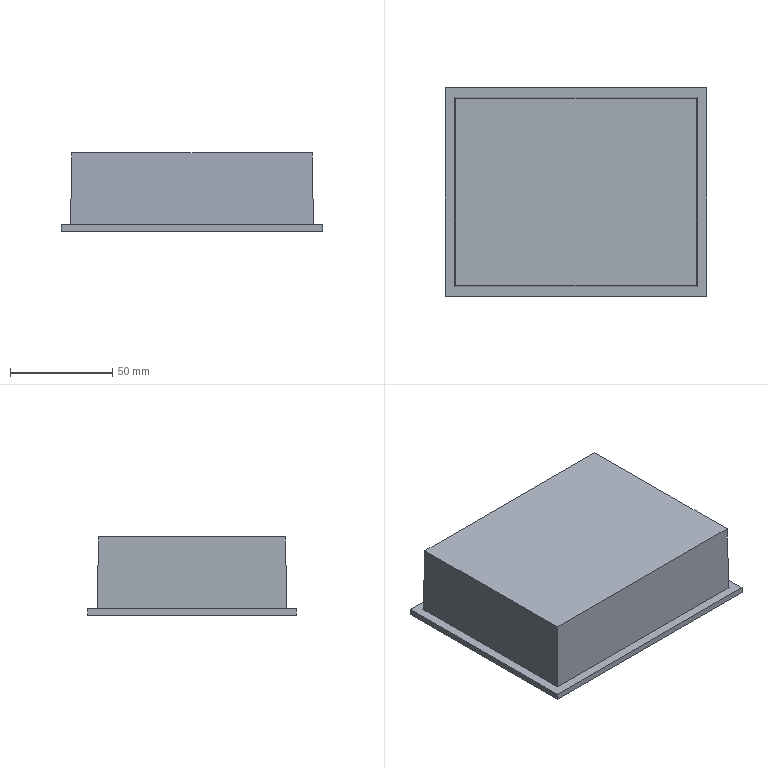Part | STEP file | Touch screen | 1 solid | 16 faces | box 128 x 102 x 38.25 mm | volume 419545 mm3 | plane 16
STEP:
#1=CARTESIAN_POINT('',(0.,0.,0.));
#2=DIRECTION('',(0.,0.,1.));
#3=DIRECTION('',(1.,0.,0.));
#4=AXIS2_PLACEMENT_3D('',#1,#2,#3);
#5=CARTESIAN_POINT('',(-64.,51.,0.));
#6=VERTEX_POINT('',#5);
#7=CARTESIAN_POINT('',(-64.,-51.,0.));
#8=VERTEX_POINT('',#7);
#9=CARTESIAN_POINT('',(-64.,51.,0.));
#10=DIRECTION('',(0.,-1.,0.));
#11=VECTOR('',#10,1.);
#12=LINE('',#9,#11);
#13=CARTESIAN_POINT('',(-64.,51.,3.));
#14=DIRECTION('',(1.,0.,0.));
#15=DIRECTION('',(0.,1.,0.));
#16=AXIS2_PLACEMENT_3D('',#13,#14,#15);
#17=PLANE('',#16);
#18=CARTESIAN_POINT('',(0.,-3.));
#19=DIRECTION('',(-1.,0.));
#20=VECTOR('',#19,1.);
#21=LINE('',#18,#20);
#22=(GEOMETRIC_REPRESENTATION_CONTEXT(2)PARAMETRIC_REPRESENTATION_CONTEXT()REPRESENTATION_CONTEXT('',''));
#23=DEFINITIONAL_REPRESENTATION('',(#21),#22);
#24=PCURVE('',#17,#23);
#25=CARTESIAN_POINT('',(0.,0.,0.));
#26=DIRECTION('',(0.,0.,-1.));
#27=DIRECTION('',(-1.,0.,0.));
#28=AXIS2_PLACEMENT_3D('',#25,#26,#27);
#29=PLANE('',#28);
#30=CARTESIAN_POINT('',(64.,51.));
#31=DIRECTION('',(0.,-1.));
#32=VECTOR('',#31,1.);
#33=LINE('',#30,#32);
#34=(GEOMETRIC_REPRESENTATION_CONTEXT(2)PARAMETRIC_REPRESENTATION_CONTEXT()REPRESENTATION_CONTEXT('',''));
#35=DEFINITIONAL_REPRESENTATION('',(#33),#34);
#36=PCURVE('',#29,#35);
#37=SURFACE_CURVE('',#12,(#24,#36),.PCURVE_S1.);
#38=EDGE_CURVE('',#6,#8,#37,.T.);
#39=ORIENTED_EDGE('',*,*,#38,.T.);
#40=CARTESIAN_POINT('',(-64.,-51.,3.));
#41=VERTEX_POINT('',#40);
#42=CARTESIAN_POINT('',(-64.,-51.,3.));
#43=DIRECTION('',(0.,0.,-1.));
#44=VECTOR('',#43,1.);
#45=LINE('',#42,#44);
#46=CARTESIAN_POINT('',(-102.,0.));
#47=DIRECTION('',(0.,-1.));
#48=VECTOR('',#47,1.);
#49=LINE('',#46,#48);
#50=(GEOMETRIC_REPRESENTATION_CONTEXT(2)PARAMETRIC_REPRESENTATION_CONTEXT()REPRESENTATION_CONTEXT('',''));
#51=DEFINITIONAL_REPRESENTATION('',(#49),#50);
#52=PCURVE('',#17,#51);
#53=CARTESIAN_POINT('',(64.,-51.,3.));
#54=DIRECTION('',(0.,1.,0.));
#55=DIRECTION('',(-1.,0.,0.));
#56=AXIS2_PLACEMENT_3D('',#53,#54,#55);
#57=PLANE('',#56);
#58=CARTESIAN_POINT('',(128.,0.));
#59=DIRECTION('',(0.,-1.));
#60=VECTOR('',#59,1.);
#61=LINE('',#58,#60);
#62=(GEOMETRIC_REPRESENTATION_CONTEXT(2)PARAMETRIC_REPRESENTATION_CONTEXT()REPRESENTATION_CONTEXT('',''));
#63=DEFINITIONAL_REPRESENTATION('',(#61),#62);
#64=PCURVE('',#57,#63);
#65=SURFACE_CURVE('',#45,(#52,#64),.PCURVE_S1.);
#66=EDGE_CURVE('',#41,#8,#65,.T.);
#67=ORIENTED_EDGE('',*,*,#66,.F.);
#68=CARTESIAN_POINT('',(-64.,51.,3.));
#69=VERTEX_POINT('',#68);
#70=CARTESIAN_POINT('',(-64.,51.,3.));
#71=DIRECTION('',(0.,-1.,0.));
#72=VECTOR('',#71,1.);
#73=LINE('',#70,#72);
#74=CARTESIAN_POINT('',(0.,0.));
#75=DIRECTION('',(-1.,0.));
#76=VECTOR('',#75,1.);
#77=LINE('',#74,#76);
#78=(GEOMETRIC_REPRESENTATION_CONTEXT(2)PARAMETRIC_REPRESENTATION_CONTEXT()REPRESENTATION_CONTEXT('',''));
#79=DEFINITIONAL_REPRESENTATION('',(#77),#78);
#80=PCURVE('',#17,#79);
#81=CARTESIAN_POINT('',(0.,0.,3.));
#82=DIRECTION('',(0.,0.,-1.));
#83=DIRECTION('',(-1.,0.,0.));
#84=AXIS2_PLACEMENT_3D('',#81,#82,#83);
#85=PLANE('',#84);
#86=CARTESIAN_POINT('',(64.,51.));
#87=DIRECTION('',(0.,-1.));
#88=VECTOR('',#87,1.);
#89=LINE('',#86,#88);
#90=(GEOMETRIC_REPRESENTATION_CONTEXT(2)PARAMETRIC_REPRESENTATION_CONTEXT()REPRESENTATION_CONTEXT('',''));
#91=DEFINITIONAL_REPRESENTATION('',(#89),#90);
#92=PCURVE('',#85,#91);
#93=SURFACE_CURVE('',#73,(#80,#92),.PCURVE_S1.);
#94=EDGE_CURVE('',#69,#41,#93,.T.);
#95=ORIENTED_EDGE('',*,*,#94,.F.);
#96=CARTESIAN_POINT('',(-64.,51.,3.));
#97=DIRECTION('',(0.,0.,-1.));
#98=VECTOR('',#97,1.);
#99=LINE('',#96,#98);
#100=CARTESIAN_POINT('',(0.,0.));
#101=DIRECTION('',(0.,-1.));
#102=VECTOR('',#101,1.);
#103=LINE('',#100,#102);
#104=(GEOMETRIC_REPRESENTATION_CONTEXT(2)PARAMETRIC_REPRESENTATION_CONTEXT()REPRESENTATION_CONTEXT('',''));
#105=DEFINITIONAL_REPRESENTATION('',(#103),#104);
#106=PCURVE('',#17,#105);
#107=CARTESIAN_POINT('',(64.,51.,3.));
#108=DIRECTION('',(0.,-1.,0.));
#109=DIRECTION('',(1.,0.,0.));
#110=AXIS2_PLACEMENT_3D('',#107,#108,#109);
#111=PLANE('',#110);
#112=CARTESIAN_POINT('',(-128.,0.));
#113=DIRECTION('',(0.,-1.));
#114=VECTOR('',#113,1.);
#115=LINE('',#112,#114);
#116=(GEOMETRIC_REPRESENTATION_CONTEXT(2)PARAMETRIC_REPRESENTATION_CONTEXT()REPRESENTATION_CONTEXT('',''));
#117=DEFINITIONAL_REPRESENTATION('',(#115),#116);
#118=PCURVE('',#111,#117);
#119=SURFACE_CURVE('',#99,(#106,#118),.PCURVE_S1.);
#120=EDGE_CURVE('',#69,#6,#119,.T.);
#121=ORIENTED_EDGE('',*,*,#120,.T.);
#122=EDGE_LOOP('',(#39,#67,#95,#121));
#123=FACE_BOUND('',#122,.T.);
#124=ADVANCED_FACE('',(#123),#17,.F.);
#125=CARTESIAN_POINT('',(64.,-51.,0.));
#126=VERTEX_POINT('',#125);
#127=CARTESIAN_POINT('',(64.,-51.,0.));
#128=DIRECTION('',(1.,0.,0.));
#129=VECTOR('',#128,1.);
#130=LINE('',#127,#129);
#131=CARTESIAN_POINT('',(0.,-3.));
#132=DIRECTION('',(-1.,0.));
#133=VECTOR('',#132,1.);
#134=LINE('',#131,#133);
#135=(GEOMETRIC_REPRESENTATION_CONTEXT(2)PARAMETRIC_REPRESENTATION_CONTEXT()REPRESENTATION_CONTEXT('',''));
#136=DEFINITIONAL_REPRESENTATION('',(#134),#135);
#137=PCURVE('',#57,#136);
#138=CARTESIAN_POINT('',(-64.,-51.));
#139=DIRECTION('',(-1.,0.));
#140=VECTOR('',#139,1.);
#141=LINE('',#138,#140);
#142=(GEOMETRIC_REPRESENTATION_CONTEXT(2)PARAMETRIC_REPRESENTATION_CONTEXT()REPRESENTATION_CONTEXT('',''));
#143=DEFINITIONAL_REPRESENTATION('',(#141),#142);
#144=PCURVE('',#29,#143);
#145=SURFACE_CURVE('',#130,(#137,#144),.PCURVE_S1.);
#146=EDGE_CURVE('',#8,#126,#145,.T.);
#147=ORIENTED_EDGE('',*,*,#146,.T.);
#148=CARTESIAN_POINT('',(64.,-51.,3.));
#149=VERTEX_POINT('',#148);
#150=CARTESIAN_POINT('',(64.,-51.,3.));
#151=DIRECTION('',(0.,0.,-1.));
#152=VECTOR('',#151,1.);
#153=LINE('',#150,#152);
#154=CARTESIAN_POINT('',(0.,0.));
#155=DIRECTION('',(0.,-1.));
#156=VECTOR('',#155,1.);
#157=LINE('',#154,#156);
#158=(GEOMETRIC_REPRESENTATION_CONTEXT(2)PARAMETRIC_REPRESENTATION_CONTEXT()REPRESENTATION_CONTEXT('',''));
#159=DEFINITIONAL_REPRESENTATION('',(#157),#158);
#160=PCURVE('',#57,#159);
#161=CARTESIAN_POINT('',(64.,51.,3.));
#162=DIRECTION('',(-1.,0.,0.));
#163=DIRECTION('',(0.,-1.,0.));
#164=AXIS2_PLACEMENT_3D('',#161,#162,#163);
#165=PLANE('',#164);
#166=CARTESIAN_POINT('',(102.,0.));
#167=DIRECTION('',(0.,-1.));
#168=VECTOR('',#167,1.);
#169=LINE('',#166,#168);
#170=(GEOMETRIC_REPRESENTATION_CONTEXT(2)PARAMETRIC_REPRESENTATION_CONTEXT()REPRESENTATION_CONTEXT('',''));
#171=DEFINITIONAL_REPRESENTATION('',(#169),#170);
#172=PCURVE('',#165,#171);
#173=SURFACE_CURVE('',#153,(#160,#172),.PCURVE_S1.);
#174=EDGE_CURVE('',#149,#126,#173,.T.);
#175=ORIENTED_EDGE('',*,*,#174,.F.);
#176=CARTESIAN_POINT('',(64.,-51.,3.));
#177=DIRECTION('',(1.,0.,0.));
#178=VECTOR('',#177,1.);
#179=LINE('',#176,#178);
#180=CARTESIAN_POINT('',(0.,0.));
#181=DIRECTION('',(-1.,0.));
#182=VECTOR('',#181,1.);
#183=LINE('',#180,#182);
#184=(GEOMETRIC_REPRESENTATION_CONTEXT(2)PARAMETRIC_REPRESENTATION_CONTEXT()REPRESENTATION_CONTEXT('',''));
#185=DEFINITIONAL_REPRESENTATION('',(#183),#184);
#186=PCURVE('',#57,#185);
#187=CARTESIAN_POINT('',(-64.,-51.));
#188=DIRECTION('',(-1.,0.));
#189=VECTOR('',#188,1.);
#190=LINE('',#187,#189);
#191=(GEOMETRIC_REPRESENTATION_CONTEXT(2)PARAMETRIC_REPRESENTATION_CONTEXT()REPRESENTATION_CONTEXT('',''));
#192=DEFINITIONAL_REPRESENTATION('',(#190),#191);
#193=PCURVE('',#85,#192);
#194=SURFACE_CURVE('',#179,(#186,#193),.PCURVE_S1.);
#195=EDGE_CURVE('',#41,#149,#194,.T.);
#196=ORIENTED_EDGE('',*,*,#195,.F.);
#197=ORIENTED_EDGE('',*,*,#66,.T.);
#198=EDGE_LOOP('',(#147,#175,#196,#197));
#199=FACE_BOUND('',#198,.T.);
#200=ADVANCED_FACE('',(#199),#57,.F.);
#201=CARTESIAN_POINT('',(64.,51.,0.));
#202=VERTEX_POINT('',#201);
#203=CARTESIAN_POINT('',(64.,51.,0.));
#204=DIRECTION('',(0.,1.,0.));
#205=VECTOR('',#204,1.);
#206=LINE('',#203,#205);
#207=CARTESIAN_POINT('',(0.,-3.));
#208=DIRECTION('',(-1.,0.));
#209=VECTOR('',#208,1.);
#210=LINE('',#207,#209);
#211=(GEOMETRIC_REPRESENTATION_CONTEXT(2)PARAMETRIC_REPRESENTATION_CONTEXT()REPRESENTATION_CONTEXT('',''));
#212=DEFINITIONAL_REPRESENTATION('',(#210),#211);
#213=PCURVE('',#165,#212);
#214=CARTESIAN_POINT('',(-64.,51.));
#215=DIRECTION('',(0.,1.));
#216=VECTOR('',#215,1.);
#217=LINE('',#214,#216);
#218=(GEOMETRIC_REPRESENTATION_CONTEXT(2)PARAMETRIC_REPRESENTATION_CONTEXT()REPRESENTATION_CONTEXT('',''));
#219=DEFINITIONAL_REPRESENTATION('',(#217),#218);
#220=PCURVE('',#29,#219);
#221=SURFACE_CURVE('',#206,(#213,#220),.PCURVE_S1.);
#222=EDGE_CURVE('',#126,#202,#221,.T.);
#223=ORIENTED_EDGE('',*,*,#222,.T.);
#224=CARTESIAN_POINT('',(64.,51.,3.));
#225=VERTEX_POINT('',#224);
#226=CARTESIAN_POINT('',(64.,51.,3.));
#227=DIRECTION('',(0.,0.,-1.));
#228=VECTOR('',#227,1.);
#229=LINE('',#226,#228);
#230=CARTESIAN_POINT('',(0.,0.));
#231=DIRECTION('',(0.,-1.));
#232=VECTOR('',#231,1.);
#233=LINE('',#230,#232);
#234=(GEOMETRIC_REPRESENTATION_CONTEXT(2)PARAMETRIC_REPRESENTATION_CONTEXT()REPRESENTATION_CONTEXT('',''));
#235=DEFINITIONAL_REPRESENTATION('',(#233),#234);
#236=PCURVE('',#165,#235);
#237=CARTESIAN_POINT('',(0.,0.));
#238=DIRECTION('',(0.,-1.));
#239=VECTOR('',#238,1.);
#240=LINE('',#237,#239);
#241=(GEOMETRIC_REPRESENTATION_CONTEXT(2)PARAMETRIC_REPRESENTATION_CONTEXT()REPRESENTATION_CONTEXT('',''));
#242=DEFINITIONAL_REPRESENTATION('',(#240),#241);
#243=PCURVE('',#111,#242);
#244=SURFACE_CURVE('',#229,(#236,#243),.PCURVE_S1.);
#245=EDGE_CURVE('',#225,#202,#244,.T.);
#246=ORIENTED_EDGE('',*,*,#245,.F.);
#247=CARTESIAN_POINT('',(64.,51.,3.));
#248=DIRECTION('',(0.,1.,0.));
#249=VECTOR('',#248,1.);
#250=LINE('',#247,#249);
#251=CARTESIAN_POINT('',(0.,0.));
#252=DIRECTION('',(-1.,0.));
#253=VECTOR('',#252,1.);
#254=LINE('',#251,#253);
#255=(GEOMETRIC_REPRESENTATION_CONTEXT(2)PARAMETRIC_REPRESENTATION_CONTEXT()REPRESENTATION_CONTEXT('',''));
#256=DEFINITIONAL_REPRESENTATION('',(#254),#255);
#257=PCURVE('',#165,#256);
#258=CARTESIAN_POINT('',(-64.,51.));
#259=DIRECTION('',(0.,1.));
#260=VECTOR('',#259,1.);
#261=LINE('',#258,#260);
#262=(GEOMETRIC_REPRESENTATION_CONTEXT(2)PARAMETRIC_REPRESENTATION_CONTEXT()REPRESENTATION_CONTEXT('',''));
#263=DEFINITIONAL_REPRESENTATION('',(#261),#262);
#264=PCURVE('',#85,#263);
#265=SURFACE_CURVE('',#250,(#257,#264),.PCURVE_S1.);
#266=EDGE_CURVE('',#149,#225,#265,.T.);
#267=ORIENTED_EDGE('',*,*,#266,.F.);
#268=ORIENTED_EDGE('',*,*,#174,.T.);
#269=EDGE_LOOP('',(#223,#246,#267,#268));
#270=FACE_BOUND('',#269,.T.);
#271=ADVANCED_FACE('',(#270),#165,.F.);
#272=CARTESIAN_POINT('',(64.,51.,0.));
#273=DIRECTION('',(-1.,0.,0.));
#274=VECTOR('',#273,1.);
#275=LINE('',#272,#274);
#276=CARTESIAN_POINT('',(0.,-3.));
#277=DIRECTION('',(-1.,0.));
#278=VECTOR('',#277,1.);
#279=LINE('',#276,#278);
#280=(GEOMETRIC_REPRESENTATION_CONTEXT(2)PARAMETRIC_REPRESENTATION_CONTEXT()REPRESENTATION_CONTEXT('',''));
#281=DEFINITIONAL_REPRESENTATION('',(#279),#280);
#282=PCURVE('',#111,#281);
#283=CARTESIAN_POINT('',(-64.,51.));
#284=DIRECTION('',(1.,0.));
#285=VECTOR('',#284,1.);
#286=LINE('',#283,#285);
#287=(GEOMETRIC_REPRESENTATION_CONTEXT(2)PARAMETRIC_REPRESENTATION_CONTEXT()REPRESENTATION_CONTEXT('',''));
#288=DEFINITIONAL_REPRESENTATION('',(#286),#287);
#289=PCURVE('',#29,#288);
#290=SURFACE_CURVE('',#275,(#282,#289),.PCURVE_S1.);
#291=EDGE_CURVE('',#202,#6,#290,.T.);
#292=ORIENTED_EDGE('',*,*,#291,.T.);
#293=ORIENTED_EDGE('',*,*,#120,.F.);
#294=CARTESIAN_POINT('',(64.,51.,3.));
#295=DIRECTION('',(-1.,0.,0.));
#296=VECTOR('',#295,1.);
#297=LINE('',#294,#296);
#298=CARTESIAN_POINT('',(0.,0.));
#299=DIRECTION('',(-1.,0.));
#300=VECTOR('',#299,1.);
#301=LINE('',#298,#300);
#302=(GEOMETRIC_REPRESENTATION_CONTEXT(2)PARAMETRIC_REPRESENTATION_CONTEXT()REPRESENTATION_CONTEXT('',''));
#303=DEFINITIONAL_REPRESENTATION('',(#301),#302);
#304=PCURVE('',#111,#303);
#305=CARTESIAN_POINT('',(-64.,51.));
#306=DIRECTION('',(1.,0.));
#307=VECTOR('',#306,1.);
#308=LINE('',#305,#307);
#309=(GEOMETRIC_REPRESENTATION_CONTEXT(2)PARAMETRIC_REPRESENTATION_CONTEXT()REPRESENTATION_CONTEXT('',''));
#310=DEFINITIONAL_REPRESENTATION('',(#308),#309);
#311=PCURVE('',#85,#310);
#312=SURFACE_CURVE('',#297,(#304,#311),.PCURVE_S1.);
#313=EDGE_CURVE('',#225,#69,#312,.T.);
#314=ORIENTED_EDGE('',*,*,#313,.F.);
#315=ORIENTED_EDGE('',*,*,#245,.T.);
#316=EDGE_LOOP('',(#292,#293,#314,#315));
#317=FACE_BOUND('',#316,.T.);
#318=ADVANCED_FACE('',(#317),#111,.F.);
#319=CARTESIAN_POINT('',(-59.5,-46.5,3.));
#320=VERTEX_POINT('',#319);
#321=CARTESIAN_POINT('',(59.5,-46.5,3.));
#322=VERTEX_POINT('',#321);
#323=CARTESIAN_POINT('',(59.5,-46.5,3.));
#324=DIRECTION('',(1.,0.,0.));
#325=VECTOR('',#324,1.);
#326=LINE('',#323,#325);
#327=CARTESIAN_POINT('',(-59.5,-46.5));
#328=DIRECTION('',(-1.,0.));
#329=VECTOR('',#328,1.);
#330=LINE('',#327,#329);
#331=(GEOMETRIC_REPRESENTATION_CONTEXT(2)PARAMETRIC_REPRESENTATION_CONTEXT()REPRESENTATION_CONTEXT('',''));
#332=DEFINITIONAL_REPRESENTATION('',(#330),#331);
#333=PCURVE('',#85,#332);
#334=CARTESIAN_POINT('',(0.,-46.542,0.9705));
#335=DIRECTION('',(0.,-0.9998,0.02085));
#336=DIRECTION('',(0.,-0.02085,-0.9998));
#337=AXIS2_PLACEMENT_3D('',#334,#335,#336);
#338=PLANE('',#337);
#339=CARTESIAN_POINT('',(-2.03,59.5));
#340=DIRECTION('',(0.,1.));
#341=VECTOR('',#340,1.);
#342=LINE('',#339,#341);
#343=(GEOMETRIC_REPRESENTATION_CONTEXT(2)PARAMETRIC_REPRESENTATION_CONTEXT()REPRESENTATION_CONTEXT('',''));
#344=DEFINITIONAL_REPRESENTATION('',(#342),#343);
#345=PCURVE('',#338,#344);
#346=SURFACE_CURVE('',#326,(#333,#345),.PCURVE_S1.);
#347=EDGE_CURVE('',#320,#322,#346,.T.);
#348=ORIENTED_EDGE('',*,*,#347,.F.);
#349=CARTESIAN_POINT('',(-59.5,46.5,3.));
#350=VERTEX_POINT('',#349);
#351=CARTESIAN_POINT('',(-59.5,46.5,3.));
#352=DIRECTION('',(0.,-1.,0.));
#353=VECTOR('',#352,1.);
#354=LINE('',#351,#353);
#355=CARTESIAN_POINT('',(59.5,46.5));
#356=DIRECTION('',(0.,-1.));
#357=VECTOR('',#356,1.);
#358=LINE('',#355,#357);
#359=(GEOMETRIC_REPRESENTATION_CONTEXT(2)PARAMETRIC_REPRESENTATION_CONTEXT()REPRESENTATION_CONTEXT('',''));
#360=DEFINITIONAL_REPRESENTATION('',(#358),#359);
#361=PCURVE('',#85,#360);
#362=CARTESIAN_POINT('',(-59.535,0.,1.072));
#363=DIRECTION('',(-0.9998,0.,0.01801));
#364=DIRECTION('',(0.01801,0.,0.9998));
#365=AXIS2_PLACEMENT_3D('',#362,#363,#364);
#366=PLANE('',#365);
#367=CARTESIAN_POINT('',(1.928,46.5));
#368=DIRECTION('',(0.,-1.));
#369=VECTOR('',#368,1.);
#370=LINE('',#367,#369);
#371=(GEOMETRIC_REPRESENTATION_CONTEXT(2)PARAMETRIC_REPRESENTATION_CONTEXT()REPRESENTATION_CONTEXT('',''));
#372=DEFINITIONAL_REPRESENTATION('',(#370),#371);
#373=PCURVE('',#366,#372);
#374=SURFACE_CURVE('',#354,(#361,#373),.PCURVE_S1.);
#375=EDGE_CURVE('',#350,#320,#374,.T.);
#376=ORIENTED_EDGE('',*,*,#375,.F.);
#377=CARTESIAN_POINT('',(59.5,46.5,3.));
#378=VERTEX_POINT('',#377);
#379=CARTESIAN_POINT('',(59.5,46.5,3.));
#380=DIRECTION('',(-1.,0.,0.));
#381=VECTOR('',#380,1.);
#382=LINE('',#379,#381);
#383=CARTESIAN_POINT('',(-59.5,46.5));
#384=DIRECTION('',(1.,0.));
#385=VECTOR('',#384,1.);
#386=LINE('',#383,#385);
#387=(GEOMETRIC_REPRESENTATION_CONTEXT(2)PARAMETRIC_REPRESENTATION_CONTEXT()REPRESENTATION_CONTEXT('',''));
#388=DEFINITIONAL_REPRESENTATION('',(#386),#387);
#389=PCURVE('',#85,#388);
#390=CARTESIAN_POINT('',(0.,46.542,0.9705));
#391=DIRECTION('',(0.,0.9998,0.02085));
#392=DIRECTION('',(0.,-0.02085,0.9998));
#393=AXIS2_PLACEMENT_3D('',#390,#391,#392);
#394=PLANE('',#393);
#395=CARTESIAN_POINT('',(2.03,59.5));
#396=DIRECTION('',(0.,-1.));
#397=VECTOR('',#396,1.);
#398=LINE('',#395,#397);
#399=(GEOMETRIC_REPRESENTATION_CONTEXT(2)PARAMETRIC_REPRESENTATION_CONTEXT()REPRESENTATION_CONTEXT('',''));
#400=DEFINITIONAL_REPRESENTATION('',(#398),#399);
#401=PCURVE('',#394,#400);
#402=SURFACE_CURVE('',#382,(#389,#401),.PCURVE_S1.);
#403=EDGE_CURVE('',#378,#350,#402,.T.);
#404=ORIENTED_EDGE('',*,*,#403,.F.);
#405=CARTESIAN_POINT('',(59.5,46.5,3.));
#406=DIRECTION('',(0.,1.,0.));
#407=VECTOR('',#406,1.);
#408=LINE('',#405,#407);
#409=CARTESIAN_POINT('',(-59.5,46.5));
#410=DIRECTION('',(0.,1.));
#411=VECTOR('',#410,1.);
#412=LINE('',#409,#411);
#413=(GEOMETRIC_REPRESENTATION_CONTEXT(2)PARAMETRIC_REPRESENTATION_CONTEXT()REPRESENTATION_CONTEXT('',''));
#414=DEFINITIONAL_REPRESENTATION('',(#412),#413);
#415=PCURVE('',#85,#414);
#416=CARTESIAN_POINT('',(59.535,0.,1.072));
#417=DIRECTION('',(0.9998,0.,0.01801));
#418=DIRECTION('',(0.01801,0.,-0.9998));
#419=AXIS2_PLACEMENT_3D('',#416,#417,#418);
#420=PLANE('',#419);
#421=CARTESIAN_POINT('',(-1.928,46.5));
#422=DIRECTION('',(0.,1.));
#423=VECTOR('',#422,1.);
#424=LINE('',#421,#423);
#425=(GEOMETRIC_REPRESENTATION_CONTEXT(2)PARAMETRIC_REPRESENTATION_CONTEXT()REPRESENTATION_CONTEXT('',''));
#426=DEFINITIONAL_REPRESENTATION('',(#424),#425);
#427=PCURVE('',#420,#426);
#428=SURFACE_CURVE('',#408,(#415,#427),.PCURVE_S1.);
#429=EDGE_CURVE('',#322,#378,#428,.T.);
#430=ORIENTED_EDGE('',*,*,#429,.F.);
#431=EDGE_LOOP('',(#348,#376,#404,#430));
#432=FACE_BOUND('',#431,.T.);
#433=ORIENTED_EDGE('',*,*,#94,.T.);
#434=ORIENTED_EDGE('',*,*,#195,.T.);
#435=ORIENTED_EDGE('',*,*,#266,.T.);
#436=ORIENTED_EDGE('',*,*,#313,.T.);
#437=EDGE_LOOP('',(#433,#434,#435,#436));
#438=FACE_BOUND('',#437,.T.);
#439=ADVANCED_FACE('',(#432,#438),#85,.F.);
#440=CARTESIAN_POINT('',(56.,41.,0.));
#441=VERTEX_POINT('',#440);
#442=CARTESIAN_POINT('',(56.,-41.,0.));
#443=VERTEX_POINT('',#442);
#444=CARTESIAN_POINT('',(56.,41.,0.));
#445=DIRECTION('',(0.,-1.,0.));
#446=VECTOR('',#445,1.);
#447=LINE('',#444,#446);
#448=CARTESIAN_POINT('',(-56.,41.));
#449=DIRECTION('',(0.,-1.));
#450=VECTOR('',#449,1.);
#451=LINE('',#448,#450);
#452=(GEOMETRIC_REPRESENTATION_CONTEXT(2)PARAMETRIC_REPRESENTATION_CONTEXT()REPRESENTATION_CONTEXT('',''));
#453=DEFINITIONAL_REPRESENTATION('',(#451),#452);
#454=PCURVE('',#29,#453);
#455=CARTESIAN_POINT('',(56.,41.,0.5));
#456=DIRECTION('',(1.,0.,0.));
#457=DIRECTION('',(0.,0.,-1.));
#458=AXIS2_PLACEMENT_3D('',#455,#456,#457);
#459=PLANE('',#458);
#460=CARTESIAN_POINT('',(0.5,0.));
#461=DIRECTION('',(0.,-1.));
#462=VECTOR('',#461,1.);
#463=LINE('',#460,#462);
#464=(GEOMETRIC_REPRESENTATION_CONTEXT(2)PARAMETRIC_REPRESENTATION_CONTEXT()REPRESENTATION_CONTEXT('',''));
#465=DEFINITIONAL_REPRESENTATION('',(#463),#464);
#466=PCURVE('',#459,#465);
#467=SURFACE_CURVE('',#447,(#454,#466),.PCURVE_S1.);
#468=EDGE_CURVE('',#441,#443,#467,.T.);
#469=ORIENTED_EDGE('',*,*,#468,.F.);
#470=CARTESIAN_POINT('',(-56.,41.,0.));
#471=VERTEX_POINT('',#470);
#472=CARTESIAN_POINT('',(-56.,41.,0.));
#473=DIRECTION('',(1.,0.,0.));
#474=VECTOR('',#473,1.);
#475=LINE('',#472,#474);
#476=CARTESIAN_POINT('',(56.,41.));
#477=DIRECTION('',(-1.,0.));
#478=VECTOR('',#477,1.);
#479=LINE('',#476,#478);
#480=(GEOMETRIC_REPRESENTATION_CONTEXT(2)PARAMETRIC_REPRESENTATION_CONTEXT()REPRESENTATION_CONTEXT('',''));
#481=DEFINITIONAL_REPRESENTATION('',(#479),#480);
#482=PCURVE('',#29,#481);
#483=CARTESIAN_POINT('',(-56.,41.,0.5));
#484=DIRECTION('',(0.,1.,0.));
#485=DIRECTION('',(0.,0.,1.));
#486=AXIS2_PLACEMENT_3D('',#483,#484,#485);
#487=PLANE('',#486);
#488=CARTESIAN_POINT('',(-0.5,0.));
#489=DIRECTION('',(0.,1.));
#490=VECTOR('',#489,1.);
#491=LINE('',#488,#490);
#492=(GEOMETRIC_REPRESENTATION_CONTEXT(2)PARAMETRIC_REPRESENTATION_CONTEXT()REPRESENTATION_CONTEXT('',''));
#493=DEFINITIONAL_REPRESENTATION('',(#491),#492);
#494=PCURVE('',#487,#493);
#495=SURFACE_CURVE('',#475,(#482,#494),.PCURVE_S1.);
#496=EDGE_CURVE('',#471,#441,#495,.T.);
#497=ORIENTED_EDGE('',*,*,#496,.F.);
#498=CARTESIAN_POINT('',(-56.,-41.,0.));
#499=VERTEX_POINT('',#498);
#500=CARTESIAN_POINT('',(-56.,41.,0.));
#501=DIRECTION('',(0.,1.,0.));
#502=VECTOR('',#501,1.);
#503=LINE('',#500,#502);
#504=CARTESIAN_POINT('',(56.,41.));
#505=DIRECTION('',(0.,1.));
#506=VECTOR('',#505,1.);
#507=LINE('',#504,#506);
#508=(GEOMETRIC_REPRESENTATION_CONTEXT(2)PARAMETRIC_REPRESENTATION_CONTEXT()REPRESENTATION_CONTEXT('',''));
#509=DEFINITIONAL_REPRESENTATION('',(#507),#508);
#510=PCURVE('',#29,#509);
#511=CARTESIAN_POINT('',(-56.,41.,0.5));
#512=DIRECTION('',(-1.,0.,0.));
#513=DIRECTION('',(0.,0.,1.));
#514=AXIS2_PLACEMENT_3D('',#511,#512,#513);
#515=PLANE('',#514);
#516=CARTESIAN_POINT('',(-0.5,0.));
#517=DIRECTION('',(0.,1.));
#518=VECTOR('',#517,1.);
#519=LINE('',#516,#518);
#520=(GEOMETRIC_REPRESENTATION_CONTEXT(2)PARAMETRIC_REPRESENTATION_CONTEXT()REPRESENTATION_CONTEXT('',''));
#521=DEFINITIONAL_REPRESENTATION('',(#519),#520);
#522=PCURVE('',#515,#521);
#523=SURFACE_CURVE('',#503,(#510,#522),.PCURVE_S1.);
#524=EDGE_CURVE('',#499,#471,#523,.T.);
#525=ORIENTED_EDGE('',*,*,#524,.F.);
#526=CARTESIAN_POINT('',(-56.,-41.,0.));
#527=DIRECTION('',(-1.,0.,0.));
#528=VECTOR('',#527,1.);
#529=LINE('',#526,#528);
#530=CARTESIAN_POINT('',(56.,-41.));
#531=DIRECTION('',(1.,0.));
#532=VECTOR('',#531,1.);
#533=LINE('',#530,#532);
#534=(GEOMETRIC_REPRESENTATION_CONTEXT(2)PARAMETRIC_REPRESENTATION_CONTEXT()REPRESENTATION_CONTEXT('',''));
#535=DEFINITIONAL_REPRESENTATION('',(#533),#534);
#536=PCURVE('',#29,#535);
#537=CARTESIAN_POINT('',(-56.,-41.,0.5));
#538=DIRECTION('',(0.,-1.,0.));
#539=DIRECTION('',(0.,0.,-1.));
#540=AXIS2_PLACEMENT_3D('',#537,#538,#539);
#541=PLANE('',#540);
#542=CARTESIAN_POINT('',(0.5,0.));
#543=DIRECTION('',(0.,-1.));
#544=VECTOR('',#543,1.);
#545=LINE('',#542,#544);
#546=(GEOMETRIC_REPRESENTATION_CONTEXT(2)PARAMETRIC_REPRESENTATION_CONTEXT()REPRESENTATION_CONTEXT('',''));
#547=DEFINITIONAL_REPRESENTATION('',(#545),#546);
#548=PCURVE('',#541,#547);
#549=SURFACE_CURVE('',#529,(#536,#548),.PCURVE_S1.);
#550=EDGE_CURVE('',#443,#499,#549,.T.);
#551=ORIENTED_EDGE('',*,*,#550,.F.);
#552=EDGE_LOOP('',(#469,#497,#525,#551));
#553=FACE_BOUND('',#552,.T.);
#554=ORIENTED_EDGE('',*,*,#38,.F.);
#555=ORIENTED_EDGE('',*,*,#291,.F.);
#556=ORIENTED_EDGE('',*,*,#222,.F.);
#557=ORIENTED_EDGE('',*,*,#146,.F.);
#558=EDGE_LOOP('',(#554,#555,#556,#557));
#559=FACE_BOUND('',#558,.T.);
#560=ADVANCED_FACE('',(#553,#559),#29,.T.);
#561=CARTESIAN_POINT('',(-58.865,45.765,38.25));
#562=VERTEX_POINT('',#561);
#563=CARTESIAN_POINT('',(-58.865,-45.765,38.25));
#564=VERTEX_POINT('',#563);
#565=CARTESIAN_POINT('',(-58.865,45.765,38.25));
#566=DIRECTION('',(0.,-1.,0.));
#567=VECTOR('',#566,1.);
#568=LINE('',#565,#567);
#569=CARTESIAN_POINT('',(0.,0.,38.25));
#570=DIRECTION('',(0.,0.,-1.));
#571=DIRECTION('',(-1.,0.,0.));
#572=AXIS2_PLACEMENT_3D('',#569,#570,#571);
#573=PLANE('',#572);
#574=CARTESIAN_POINT('',(58.865,45.765));
#575=DIRECTION('',(0.,-1.));
#576=VECTOR('',#575,1.);
#577=LINE('',#574,#576);
#578=(GEOMETRIC_REPRESENTATION_CONTEXT(2)PARAMETRIC_REPRESENTATION_CONTEXT()REPRESENTATION_CONTEXT('',''));
#579=DEFINITIONAL_REPRESENTATION('',(#577),#578);
#580=PCURVE('',#573,#579);
#581=CARTESIAN_POINT('',(37.184,45.765));
#582=DIRECTION('',(0.,-1.));
#583=VECTOR('',#582,1.);
#584=LINE('',#581,#583);
#585=(GEOMETRIC_REPRESENTATION_CONTEXT(2)PARAMETRIC_REPRESENTATION_CONTEXT()REPRESENTATION_CONTEXT('',''));
#586=DEFINITIONAL_REPRESENTATION('',(#584),#585);
#587=PCURVE('',#366,#586);
#588=SURFACE_CURVE('',#568,(#580,#587),.PCURVE_S1.);
#589=EDGE_CURVE('',#562,#564,#588,.T.);
#590=ORIENTED_EDGE('',*,*,#589,.T.);
#591=CARTESIAN_POINT('',(58.865,-45.765,38.25));
#592=VERTEX_POINT('',#591);
#593=CARTESIAN_POINT('',(58.865,-45.765,38.25));
#594=DIRECTION('',(1.,0.,0.));
#595=VECTOR('',#594,1.);
#596=LINE('',#593,#595);
#597=CARTESIAN_POINT('',(-58.865,-45.765));
#598=DIRECTION('',(-1.,0.));
#599=VECTOR('',#598,1.);
#600=LINE('',#597,#599);
#601=(GEOMETRIC_REPRESENTATION_CONTEXT(2)PARAMETRIC_REPRESENTATION_CONTEXT()REPRESENTATION_CONTEXT('',''));
#602=DEFINITIONAL_REPRESENTATION('',(#600),#601);
#603=PCURVE('',#573,#602);
#604=CARTESIAN_POINT('',(-37.288,58.865));
#605=DIRECTION('',(0.,1.));
#606=VECTOR('',#605,1.);
#607=LINE('',#604,#606);
#608=(GEOMETRIC_REPRESENTATION_CONTEXT(2)PARAMETRIC_REPRESENTATION_CONTEXT()REPRESENTATION_CONTEXT('',''));
#609=DEFINITIONAL_REPRESENTATION('',(#607),#608);
#610=PCURVE('',#338,#609);
#611=SURFACE_CURVE('',#596,(#603,#610),.PCURVE_S1.);
#612=EDGE_CURVE('',#564,#592,#611,.T.);
#613=ORIENTED_EDGE('',*,*,#612,.T.);
#614=CARTESIAN_POINT('',(58.865,45.765,38.25));
#615=VERTEX_POINT('',#614);
#616=CARTESIAN_POINT('',(58.865,45.765,38.25));
#617=DIRECTION('',(0.,1.,0.));
#618=VECTOR('',#617,1.);
#619=LINE('',#616,#618);
#620=CARTESIAN_POINT('',(-58.865,45.765));
#621=DIRECTION('',(0.,1.));
#622=VECTOR('',#621,1.);
#623=LINE('',#620,#622);
#624=(GEOMETRIC_REPRESENTATION_CONTEXT(2)PARAMETRIC_REPRESENTATION_CONTEXT()REPRESENTATION_CONTEXT('',''));
#625=DEFINITIONAL_REPRESENTATION('',(#623),#624);
#626=PCURVE('',#573,#625);
#627=CARTESIAN_POINT('',(-37.184,45.765));
#628=DIRECTION('',(0.,1.));
#629=VECTOR('',#628,1.);
#630=LINE('',#627,#629);
#631=(GEOMETRIC_REPRESENTATION_CONTEXT(2)PARAMETRIC_REPRESENTATION_CONTEXT()REPRESENTATION_CONTEXT('',''));
#632=DEFINITIONAL_REPRESENTATION('',(#630),#631);
#633=PCURVE('',#420,#632);
#634=SURFACE_CURVE('',#619,(#626,#633),.PCURVE_S1.);
#635=EDGE_CURVE('',#592,#615,#634,.T.);
#636=ORIENTED_EDGE('',*,*,#635,.T.);
#637=CARTESIAN_POINT('',(58.865,45.765,38.25));
#638=DIRECTION('',(-1.,0.,0.));
#639=VECTOR('',#638,1.);
#640=LINE('',#637,#639);
#641=CARTESIAN_POINT('',(-58.865,45.765));
#642=DIRECTION('',(1.,0.));
#643=VECTOR('',#642,1.);
#644=LINE('',#641,#643);
#645=(GEOMETRIC_REPRESENTATION_CONTEXT(2)PARAMETRIC_REPRESENTATION_CONTEXT()REPRESENTATION_CONTEXT('',''));
#646=DEFINITIONAL_REPRESENTATION('',(#644),#645);
#647=PCURVE('',#573,#646);
#648=CARTESIAN_POINT('',(37.288,58.865));
#649=DIRECTION('',(0.,-1.));
#650=VECTOR('',#649,1.);
#651=LINE('',#648,#650);
#652=(GEOMETRIC_REPRESENTATION_CONTEXT(2)PARAMETRIC_REPRESENTATION_CONTEXT()REPRESENTATION_CONTEXT('',''));
#653=DEFINITIONAL_REPRESENTATION('',(#651),#652);
#654=PCURVE('',#394,#653);
#655=SURFACE_CURVE('',#640,(#647,#654),.PCURVE_S1.);
#656=EDGE_CURVE('',#615,#562,#655,.T.);
#657=ORIENTED_EDGE('',*,*,#656,.T.);
#658=EDGE_LOOP('',(#590,#613,#636,#657));
#659=FACE_BOUND('',#658,.T.);
#660=ADVANCED_FACE('',(#659),#573,.F.);
#661=CARTESIAN_POINT('',(58.865,-45.765,38.25));
#662=DIRECTION('',(0.01801,-0.02084,-0.9996));
#663=VECTOR('',#662,1.);
#664=LINE('',#661,#663);
#665=CARTESIAN_POINT('',(-37.184,-45.765));
#666=DIRECTION('',(0.9998,-0.02084));
#667=VECTOR('',#666,1.);
#668=LINE('',#665,#667);
#669=(GEOMETRIC_REPRESENTATION_CONTEXT(2)PARAMETRIC_REPRESENTATION_CONTEXT()REPRESENTATION_CONTEXT('',''));
#670=DEFINITIONAL_REPRESENTATION('',(#668),#669);
#671=PCURVE('',#420,#670);
#672=CARTESIAN_POINT('',(-37.288,58.865));
#673=DIRECTION('',(0.9998,0.01801));
#674=VECTOR('',#673,1.);
#675=LINE('',#672,#674);
#676=(GEOMETRIC_REPRESENTATION_CONTEXT(2)PARAMETRIC_REPRESENTATION_CONTEXT()REPRESENTATION_CONTEXT('',''));
#677=DEFINITIONAL_REPRESENTATION('',(#675),#676);
#678=PCURVE('',#338,#677);
#679=SURFACE_CURVE('',#664,(#671,#678),.PCURVE_S1.);
#680=EDGE_CURVE('',#592,#322,#679,.T.);
#681=ORIENTED_EDGE('',*,*,#680,.T.);
#682=ORIENTED_EDGE('',*,*,#429,.T.);
#683=CARTESIAN_POINT('',(58.865,45.765,38.25));
#684=DIRECTION('',(0.01801,0.02084,-0.9996));
#685=VECTOR('',#684,1.);
#686=LINE('',#683,#685);
#687=CARTESIAN_POINT('',(-37.184,45.765));
#688=DIRECTION('',(0.9998,0.02084));
#689=VECTOR('',#688,1.);
#690=LINE('',#687,#689);
#691=(GEOMETRIC_REPRESENTATION_CONTEXT(2)PARAMETRIC_REPRESENTATION_CONTEXT()REPRESENTATION_CONTEXT('',''));
#692=DEFINITIONAL_REPRESENTATION('',(#690),#691);
#693=PCURVE('',#420,#692);
#694=CARTESIAN_POINT('',(37.288,58.865));
#695=DIRECTION('',(-0.9998,0.01801));
#696=VECTOR('',#695,1.);
#697=LINE('',#694,#696);
#698=(GEOMETRIC_REPRESENTATION_CONTEXT(2)PARAMETRIC_REPRESENTATION_CONTEXT()REPRESENTATION_CONTEXT('',''));
#699=DEFINITIONAL_REPRESENTATION('',(#697),#698);
#700=PCURVE('',#394,#699);
#701=SURFACE_CURVE('',#686,(#693,#700),.PCURVE_S1.);
#702=EDGE_CURVE('',#615,#378,#701,.T.);
#703=ORIENTED_EDGE('',*,*,#702,.F.);
#704=ORIENTED_EDGE('',*,*,#635,.F.);
#705=EDGE_LOOP('',(#681,#682,#703,#704));
#706=FACE_BOUND('',#705,.T.);
#707=ADVANCED_FACE('',(#706),#420,.T.);
#708=ORIENTED_EDGE('',*,*,#702,.T.);
#709=ORIENTED_EDGE('',*,*,#403,.T.);
#710=CARTESIAN_POINT('',(-58.865,45.765,38.25));
#711=DIRECTION('',(-0.01801,0.02084,-0.9996));
#712=VECTOR('',#711,1.);
#713=LINE('',#710,#712);
#714=CARTESIAN_POINT('',(37.288,-58.865));
#715=DIRECTION('',(-0.9998,-0.01801));
#716=VECTOR('',#715,1.);
#717=LINE('',#714,#716);
#718=(GEOMETRIC_REPRESENTATION_CONTEXT(2)PARAMETRIC_REPRESENTATION_CONTEXT()REPRESENTATION_CONTEXT('',''));
#719=DEFINITIONAL_REPRESENTATION('',(#717),#718);
#720=PCURVE('',#394,#719);
#721=CARTESIAN_POINT('',(37.184,45.765));
#722=DIRECTION('',(-0.9998,0.02084));
#723=VECTOR('',#722,1.);
#724=LINE('',#721,#723);
#725=(GEOMETRIC_REPRESENTATION_CONTEXT(2)PARAMETRIC_REPRESENTATION_CONTEXT()REPRESENTATION_CONTEXT('',''));
#726=DEFINITIONAL_REPRESENTATION('',(#724),#725);
#727=PCURVE('',#366,#726);
#728=SURFACE_CURVE('',#713,(#720,#727),.PCURVE_S1.);
#729=EDGE_CURVE('',#562,#350,#728,.T.);
#730=ORIENTED_EDGE('',*,*,#729,.F.);
#731=ORIENTED_EDGE('',*,*,#656,.F.);
#732=EDGE_LOOP('',(#708,#709,#730,#731));
#733=FACE_BOUND('',#732,.T.);
#734=ADVANCED_FACE('',(#733),#394,.T.);
#735=CARTESIAN_POINT('',(-58.865,-45.765,38.25));
#736=DIRECTION('',(-0.01801,-0.02084,-0.9996));
#737=VECTOR('',#736,1.);
#738=LINE('',#735,#737);
#739=CARTESIAN_POINT('',(-37.288,-58.865));
#740=DIRECTION('',(0.9998,-0.01801));
#741=VECTOR('',#740,1.);
#742=LINE('',#739,#741);
#743=(GEOMETRIC_REPRESENTATION_CONTEXT(2)PARAMETRIC_REPRESENTATION_CONTEXT()REPRESENTATION_CONTEXT('',''));
#744=DEFINITIONAL_REPRESENTATION('',(#742),#743);
#745=PCURVE('',#338,#744);
#746=CARTESIAN_POINT('',(37.184,-45.765));
#747=DIRECTION('',(-0.9998,-0.02084));
#748=VECTOR('',#747,1.);
#749=LINE('',#746,#748);
#750=(GEOMETRIC_REPRESENTATION_CONTEXT(2)PARAMETRIC_REPRESENTATION_CONTEXT()REPRESENTATION_CONTEXT('',''));
#751=DEFINITIONAL_REPRESENTATION('',(#749),#750);
#752=PCURVE('',#366,#751);
#753=SURFACE_CURVE('',#738,(#745,#752),.PCURVE_S1.);
#754=EDGE_CURVE('',#564,#320,#753,.T.);
#755=ORIENTED_EDGE('',*,*,#754,.T.);
#756=ORIENTED_EDGE('',*,*,#347,.T.);
#757=ORIENTED_EDGE('',*,*,#680,.F.);
#758=ORIENTED_EDGE('',*,*,#612,.F.);
#759=EDGE_LOOP('',(#755,#756,#757,#758));
#760=FACE_BOUND('',#759,.T.);
#761=ADVANCED_FACE('',(#760),#338,.T.);
#762=ORIENTED_EDGE('',*,*,#729,.T.);
#763=ORIENTED_EDGE('',*,*,#375,.T.);
#764=ORIENTED_EDGE('',*,*,#754,.F.);
#765=ORIENTED_EDGE('',*,*,#589,.F.);
#766=EDGE_LOOP('',(#762,#763,#764,#765));
#767=FACE_BOUND('',#766,.T.);
#768=ADVANCED_FACE('',(#767),#366,.T.);
#769=ORIENTED_EDGE('',*,*,#468,.T.);
#770=CARTESIAN_POINT('',(56.,-41.,0.5));
#771=VERTEX_POINT('',#770);
#772=CARTESIAN_POINT('',(56.,-41.,0.5));
#773=DIRECTION('',(0.,0.,-1.));
#774=VECTOR('',#773,1.);
#775=LINE('',#772,#774);
#776=CARTESIAN_POINT('',(0.,-82.));
#777=DIRECTION('',(1.,0.));
#778=VECTOR('',#777,1.);
#779=LINE('',#776,#778);
#780=(GEOMETRIC_REPRESENTATION_CONTEXT(2)PARAMETRIC_REPRESENTATION_CONTEXT()REPRESENTATION_CONTEXT('',''));
#781=DEFINITIONAL_REPRESENTATION('',(#779),#780);
#782=PCURVE('',#459,#781);
#783=CARTESIAN_POINT('',(0.,112.));
#784=DIRECTION('',(1.,0.));
#785=VECTOR('',#784,1.);
#786=LINE('',#783,#785);
#787=(GEOMETRIC_REPRESENTATION_CONTEXT(2)PARAMETRIC_REPRESENTATION_CONTEXT()REPRESENTATION_CONTEXT('',''));
#788=DEFINITIONAL_REPRESENTATION('',(#786),#787);
#789=PCURVE('',#541,#788);
#790=SURFACE_CURVE('',#775,(#782,#789),.PCURVE_S1.);
#791=EDGE_CURVE('',#771,#443,#790,.T.);
#792=ORIENTED_EDGE('',*,*,#791,.F.);
#793=CARTESIAN_POINT('',(56.,41.,0.5));
#794=VERTEX_POINT('',#793);
#795=CARTESIAN_POINT('',(56.,41.,0.5));
#796=DIRECTION('',(0.,-1.,0.));
#797=VECTOR('',#796,1.);
#798=LINE('',#795,#797);
#799=CARTESIAN_POINT('',(0.,0.));
#800=DIRECTION('',(0.,-1.));
#801=VECTOR('',#800,1.);
#802=LINE('',#799,#801);
#803=(GEOMETRIC_REPRESENTATION_CONTEXT(2)PARAMETRIC_REPRESENTATION_CONTEXT()REPRESENTATION_CONTEXT('',''));
#804=DEFINITIONAL_REPRESENTATION('',(#802),#803);
#805=PCURVE('',#459,#804);
#806=CARTESIAN_POINT('',(0.,0.,0.5));
#807=DIRECTION('',(0.,0.,1.));
#808=DIRECTION('',(1.,0.,0.));
#809=AXIS2_PLACEMENT_3D('',#806,#807,#808);
#810=PLANE('',#809);
#811=CARTESIAN_POINT('',(56.,41.));
#812=DIRECTION('',(0.,-1.));
#813=VECTOR('',#812,1.);
#814=LINE('',#811,#813);
#815=(GEOMETRIC_REPRESENTATION_CONTEXT(2)PARAMETRIC_REPRESENTATION_CONTEXT()REPRESENTATION_CONTEXT('',''));
#816=DEFINITIONAL_REPRESENTATION('',(#814),#815);
#817=PCURVE('',#810,#816);
#818=SURFACE_CURVE('',#798,(#805,#817),.PCURVE_S1.);
#819=EDGE_CURVE('',#794,#771,#818,.T.);
#820=ORIENTED_EDGE('',*,*,#819,.F.);
#821=CARTESIAN_POINT('',(56.,41.,0.5));
#822=DIRECTION('',(0.,0.,-1.));
#823=VECTOR('',#822,1.);
#824=LINE('',#821,#823);
#825=CARTESIAN_POINT('',(0.,0.));
#826=DIRECTION('',(1.,0.));
#827=VECTOR('',#826,1.);
#828=LINE('',#825,#827);
#829=(GEOMETRIC_REPRESENTATION_CONTEXT(2)PARAMETRIC_REPRESENTATION_CONTEXT()REPRESENTATION_CONTEXT('',''));
#830=DEFINITIONAL_REPRESENTATION('',(#828),#829);
#831=PCURVE('',#459,#830);
#832=CARTESIAN_POINT('',(0.,112.));
#833=DIRECTION('',(-1.,0.));
#834=VECTOR('',#833,1.);
#835=LINE('',#832,#834);
#836=(GEOMETRIC_REPRESENTATION_CONTEXT(2)PARAMETRIC_REPRESENTATION_CONTEXT()REPRESENTATION_CONTEXT('',''));
#837=DEFINITIONAL_REPRESENTATION('',(#835),#836);
#838=PCURVE('',#487,#837);
#839=SURFACE_CURVE('',#824,(#831,#838),.PCURVE_S1.);
#840=EDGE_CURVE('',#794,#441,#839,.T.);
#841=ORIENTED_EDGE('',*,*,#840,.T.);
#842=EDGE_LOOP('',(#769,#792,#820,#841));
#843=FACE_BOUND('',#842,.T.);
#844=ADVANCED_FACE('',(#843),#459,.F.);
#845=ORIENTED_EDGE('',*,*,#496,.T.);
#846=ORIENTED_EDGE('',*,*,#840,.F.);
#847=CARTESIAN_POINT('',(-56.,41.,0.5));
#848=VERTEX_POINT('',#847);
#849=CARTESIAN_POINT('',(-56.,41.,0.5));
#850=DIRECTION('',(1.,0.,0.));
#851=VECTOR('',#850,1.);
#852=LINE('',#849,#851);
#853=CARTESIAN_POINT('',(0.,0.));
#854=DIRECTION('',(0.,1.));
#855=VECTOR('',#854,1.);
#856=LINE('',#853,#855);
#857=(GEOMETRIC_REPRESENTATION_CONTEXT(2)PARAMETRIC_REPRESENTATION_CONTEXT()REPRESENTATION_CONTEXT('',''));
#858=DEFINITIONAL_REPRESENTATION('',(#856),#857);
#859=PCURVE('',#487,#858);
#860=CARTESIAN_POINT('',(-56.,41.));
#861=DIRECTION('',(1.,0.));
#862=VECTOR('',#861,1.);
#863=LINE('',#860,#862);
#864=(GEOMETRIC_REPRESENTATION_CONTEXT(2)PARAMETRIC_REPRESENTATION_CONTEXT()REPRESENTATION_CONTEXT('',''));
#865=DEFINITIONAL_REPRESENTATION('',(#863),#864);
#866=PCURVE('',#810,#865);
#867=SURFACE_CURVE('',#852,(#859,#866),.PCURVE_S1.);
#868=EDGE_CURVE('',#848,#794,#867,.T.);
#869=ORIENTED_EDGE('',*,*,#868,.F.);
#870=CARTESIAN_POINT('',(-56.,41.,0.5));
#871=DIRECTION('',(0.,0.,-1.));
#872=VECTOR('',#871,1.);
#873=LINE('',#870,#872);
#874=CARTESIAN_POINT('',(0.,0.));
#875=DIRECTION('',(-1.,0.));
#876=VECTOR('',#875,1.);
#877=LINE('',#874,#876);
#878=(GEOMETRIC_REPRESENTATION_CONTEXT(2)PARAMETRIC_REPRESENTATION_CONTEXT()REPRESENTATION_CONTEXT('',''));
#879=DEFINITIONAL_REPRESENTATION('',(#877),#878);
#880=PCURVE('',#487,#879);
#881=CARTESIAN_POINT('',(0.,0.));
#882=DIRECTION('',(-1.,0.));
#883=VECTOR('',#882,1.);
#884=LINE('',#881,#883);
#885=(GEOMETRIC_REPRESENTATION_CONTEXT(2)PARAMETRIC_REPRESENTATION_CONTEXT()REPRESENTATION_CONTEXT('',''));
#886=DEFINITIONAL_REPRESENTATION('',(#884),#885);
#887=PCURVE('',#515,#886);
#888=SURFACE_CURVE('',#873,(#880,#887),.PCURVE_S1.);
#889=EDGE_CURVE('',#848,#471,#888,.T.);
#890=ORIENTED_EDGE('',*,*,#889,.T.);
#891=EDGE_LOOP('',(#845,#846,#869,#890));
#892=FACE_BOUND('',#891,.T.);
#893=ADVANCED_FACE('',(#892),#487,.F.);
#894=ORIENTED_EDGE('',*,*,#524,.T.);
#895=ORIENTED_EDGE('',*,*,#889,.F.);
#896=CARTESIAN_POINT('',(-56.,-41.,0.5));
#897=VERTEX_POINT('',#896);
#898=CARTESIAN_POINT('',(-56.,41.,0.5));
#899=DIRECTION('',(0.,1.,0.));
#900=VECTOR('',#899,1.);
#901=LINE('',#898,#900);
#902=CARTESIAN_POINT('',(0.,0.));
#903=DIRECTION('',(0.,1.));
#904=VECTOR('',#903,1.);
#905=LINE('',#902,#904);
#906=(GEOMETRIC_REPRESENTATION_CONTEXT(2)PARAMETRIC_REPRESENTATION_CONTEXT()REPRESENTATION_CONTEXT('',''));
#907=DEFINITIONAL_REPRESENTATION('',(#905),#906);
#908=PCURVE('',#515,#907);
#909=CARTESIAN_POINT('',(-56.,41.));
#910=DIRECTION('',(0.,1.));
#911=VECTOR('',#910,1.);
#912=LINE('',#909,#911);
#913=(GEOMETRIC_REPRESENTATION_CONTEXT(2)PARAMETRIC_REPRESENTATION_CONTEXT()REPRESENTATION_CONTEXT('',''));
#914=DEFINITIONAL_REPRESENTATION('',(#912),#913);
#915=PCURVE('',#810,#914);
#916=SURFACE_CURVE('',#901,(#908,#915),.PCURVE_S1.);
#917=EDGE_CURVE('',#897,#848,#916,.T.);
#918=ORIENTED_EDGE('',*,*,#917,.F.);
#919=CARTESIAN_POINT('',(-56.,-41.,0.5));
#920=DIRECTION('',(0.,0.,-1.));
#921=VECTOR('',#920,1.);
#922=LINE('',#919,#921);
#923=CARTESIAN_POINT('',(0.,-82.));
#924=DIRECTION('',(-1.,0.));
#925=VECTOR('',#924,1.);
#926=LINE('',#923,#925);
#927=(GEOMETRIC_REPRESENTATION_CONTEXT(2)PARAMETRIC_REPRESENTATION_CONTEXT()REPRESENTATION_CONTEXT('',''));
#928=DEFINITIONAL_REPRESENTATION('',(#926),#927);
#929=PCURVE('',#515,#928);
#930=CARTESIAN_POINT('',(0.,0.));
#931=DIRECTION('',(1.,0.));
#932=VECTOR('',#931,1.);
#933=LINE('',#930,#932);
#934=(GEOMETRIC_REPRESENTATION_CONTEXT(2)PARAMETRIC_REPRESENTATION_CONTEXT()REPRESENTATION_CONTEXT('',''));
#935=DEFINITIONAL_REPRESENTATION('',(#933),#934);
#936=PCURVE('',#541,#935);
#937=SURFACE_CURVE('',#922,(#929,#936),.PCURVE_S1.);
#938=EDGE_CURVE('',#897,#499,#937,.T.);
#939=ORIENTED_EDGE('',*,*,#938,.T.);
#940=EDGE_LOOP('',(#894,#895,#918,#939));
#941=FACE_BOUND('',#940,.T.);
#942=ADVANCED_FACE('',(#941),#515,.F.);
#943=ORIENTED_EDGE('',*,*,#550,.T.);
#944=ORIENTED_EDGE('',*,*,#938,.F.);
#945=CARTESIAN_POINT('',(-56.,-41.,0.5));
#946=DIRECTION('',(-1.,0.,0.));
#947=VECTOR('',#946,1.);
#948=LINE('',#945,#947);
#949=CARTESIAN_POINT('',(0.,0.));
#950=DIRECTION('',(0.,-1.));
#951=VECTOR('',#950,1.);
#952=LINE('',#949,#951);
#953=(GEOMETRIC_REPRESENTATION_CONTEXT(2)PARAMETRIC_REPRESENTATION_CONTEXT()REPRESENTATION_CONTEXT('',''));
#954=DEFINITIONAL_REPRESENTATION('',(#952),#953);
#955=PCURVE('',#541,#954);
#956=CARTESIAN_POINT('',(-56.,-41.));
#957=DIRECTION('',(-1.,0.));
#958=VECTOR('',#957,1.);
#959=LINE('',#956,#958);
#960=(GEOMETRIC_REPRESENTATION_CONTEXT(2)PARAMETRIC_REPRESENTATION_CONTEXT()REPRESENTATION_CONTEXT('',''));
#961=DEFINITIONAL_REPRESENTATION('',(#959),#960);
#962=PCURVE('',#810,#961);
#963=SURFACE_CURVE('',#948,(#955,#962),.PCURVE_S1.);
#964=EDGE_CURVE('',#771,#897,#963,.T.);
#965=ORIENTED_EDGE('',*,*,#964,.F.);
#966=ORIENTED_EDGE('',*,*,#791,.T.);
#967=EDGE_LOOP('',(#943,#944,#965,#966));
#968=FACE_BOUND('',#967,.T.);
#969=ADVANCED_FACE('',(#968),#541,.F.);
#970=ORIENTED_EDGE('',*,*,#819,.T.);
#971=ORIENTED_EDGE('',*,*,#964,.T.);
#972=ORIENTED_EDGE('',*,*,#917,.T.);
#973=ORIENTED_EDGE('',*,*,#868,.T.);
#974=EDGE_LOOP('',(#970,#971,#972,#973));
#975=FACE_BOUND('',#974,.T.);
#976=ADVANCED_FACE('',(#975),#810,.F.);
#977=CLOSED_SHELL('',(#124,#200,#271,#318,#439,#560,#660,#707,#734,#761,#768,#844,#893,#942,#969,#976));
#978=MANIFOLD_SOLID_BREP('',#977);
#979=(LENGTH_UNIT()NAMED_UNIT(*)SI_UNIT(.MILLI.,.METRE.));
#980=UNCERTAINTY_MEASURE_WITH_UNIT(LENGTH_MEASURE(0.0000001),#979,'','');
#981=(NAMED_UNIT(*)PLANE_ANGLE_UNIT()SI_UNIT($,.RADIAN.));
#982=(NAMED_UNIT(*)SI_UNIT($,.STERADIAN.)SOLID_ANGLE_UNIT());
#983=(GEOMETRIC_REPRESENTATION_CONTEXT(3)GLOBAL_UNCERTAINTY_ASSIGNED_CONTEXT((#980))GLOBAL_UNIT_ASSIGNED_CONTEXT((#979,#981,#982))REPRESENTATION_CONTEXT('',''));
#984=ADVANCED_BREP_SHAPE_REPRESENTATION('',(#4,#978),#983);